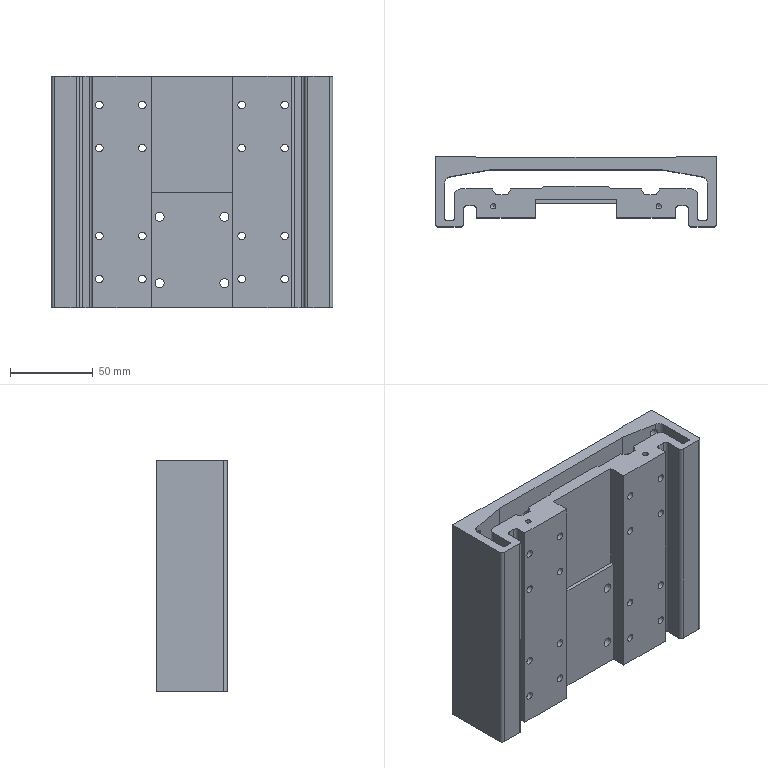Part | STEP file | 1 solid | 162 faces | box 170 x 42.5 x 140 mm | volume 522527 mm3 | cylinder 86 | plane 72 | cone 4 | commonest cylinder face diameters 8 x36 4.5 x16 4 x8 9 x8 2 x4 3.3 x4